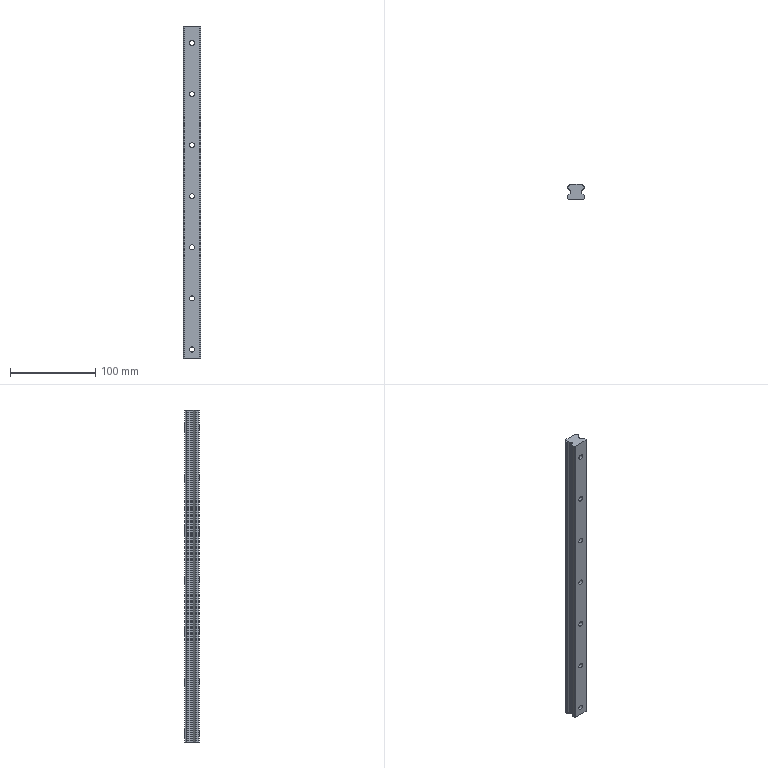Part | STEP file | P-008244^LM06S-05-03-02B | 1 solid | 79 faces | box 20 x 17.5 x 390 mm | volume 110981 mm3 | cylinder 50 | plane 29 | commonest cylinder face diameters 6 x14 9.5 x14 1 x12 2 x6 4.06 x4